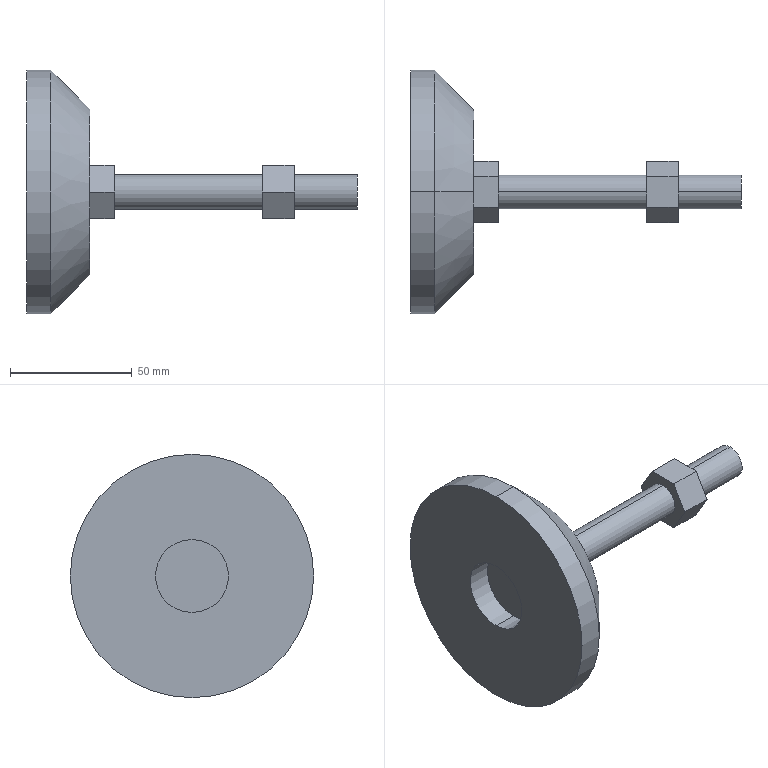Part | STEP file | Foot | 1 solid | 29 faces | box 136 x 100 x 100 mm | volume 184245 mm3 | plane 19 | cylinder 8 | cone 2 | commonest cylinder face diameters 14 x4 30 x2 100 x2